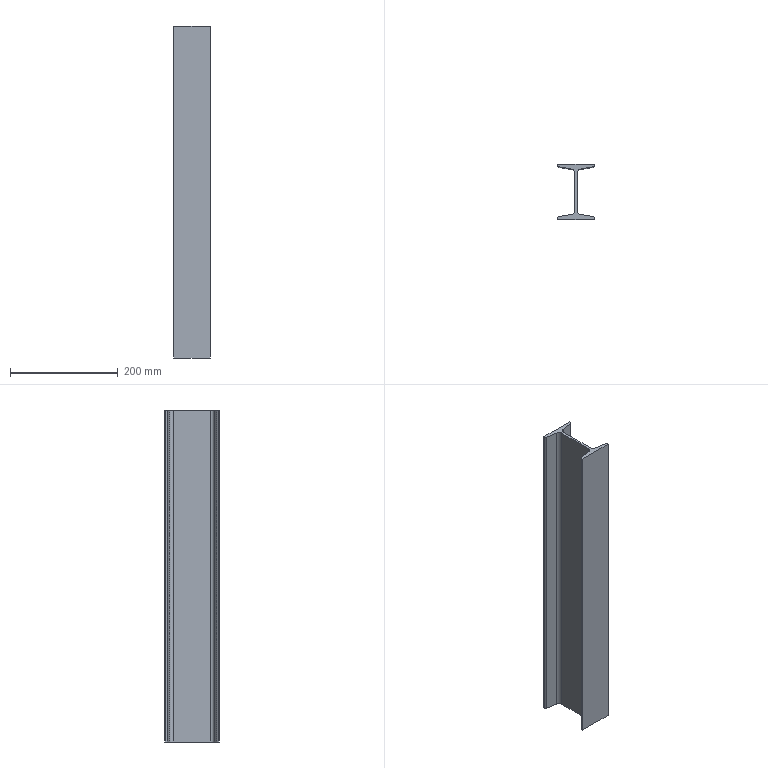Part | SolidWorks | features BaseBody 1 | 1 solid | 22 faces | box 67.6 x 101.6 x 617.6 mm | volume 858414 mm3 | plane 14 | cylinder 8 | commonest cylinder face diameters 5.6 x4 14.8 x4
STEP:
#1=CARTESIAN_POINT('',(9.458,64.672,0.));
#2=VERTEX_POINT('',#1);
#3=CARTESIAN_POINT('',(9.458,-5.208,0.));
#4=VERTEX_POINT('',#3);
#5=CARTESIAN_POINT('',(9.458,-5.208,0.));
#6=DIRECTION('',(0.,-1.,0.));
#7=VECTOR('',#6,1000.);
#8=LINE('',#5,#7);
#9=EDGE_CURVE('',#2,#4,#8,.T.);
#10=ORIENTED_EDGE('',*,*,#9,.T.);
#11=CARTESIAN_POINT('',(9.458,-5.208,617.6));
#12=VERTEX_POINT('',#11);
#13=CARTESIAN_POINT('',(9.458,-5.208,0.));
#14=DIRECTION('',(0.,0.,1.));
#15=VECTOR('',#14,1000.);
#16=LINE('',#13,#15);
#17=EDGE_CURVE('',#4,#12,#16,.T.);
#18=ORIENTED_EDGE('',*,*,#17,.T.);
#19=CARTESIAN_POINT('',(9.458,64.672,617.6));
#20=VERTEX_POINT('',#19);
#21=CARTESIAN_POINT('',(9.458,-5.208,617.6));
#22=DIRECTION('',(0.,1.,0.));
#23=VECTOR('',#22,1000.);
#24=LINE('',#21,#23);
#25=EDGE_CURVE('',#12,#20,#24,.T.);
#26=ORIENTED_EDGE('',*,*,#25,.T.);
#27=CARTESIAN_POINT('',(9.458,64.672,0.));
#28=DIRECTION('',(0.,0.,-1.));
#29=VECTOR('',#28,1000.);
#30=LINE('',#27,#29);
#31=EDGE_CURVE('',#20,#2,#30,.T.);
#32=ORIENTED_EDGE('',*,*,#31,.T.);
#33=EDGE_LOOP('',(#10,#18,#26,#32));
#34=FACE_OUTER_BOUND('',#33,.T.);
#35=CARTESIAN_POINT('',(9.458,-5.208,0.));
#36=DIRECTION('',(-1.,0.,0.));
#37=DIRECTION('',(0.,0.,1.));
#38=AXIS2_PLACEMENT_3D('',#35,#36,#37);
#39=PLANE('',#38);
#40=ADVANCED_FACE('',(#34),#39,.T.);
#41=ORIENTED_EDGE('',*,*,#17,.F.);
#42=CARTESIAN_POINT('',(3.279,-12.506,0.));
#43=VERTEX_POINT('',#42);
#44=CARTESIAN_POINT('',(2.058,-5.208,0.));
#45=DIRECTION('',(0.,0.,1.));
#46=DIRECTION('',(1.,0.,0.));
#47=AXIS2_PLACEMENT_3D('',#44,#45,#46);
#48=CIRCLE('',#47,7.4);
#49=EDGE_CURVE('',#43,#4,#48,.T.);
#50=ORIENTED_EDGE('',*,*,#49,.F.);
#51=CARTESIAN_POINT('',(3.279,-12.506,617.6));
#52=VERTEX_POINT('',#51);
#53=CARTESIAN_POINT('',(3.279,-12.506,0.));
#54=DIRECTION('',(0.,0.,-1.));
#55=VECTOR('',#54,1000.);
#56=LINE('',#53,#55);
#57=EDGE_CURVE('',#52,#43,#56,.T.);
#58=ORIENTED_EDGE('',*,*,#57,.F.);
#59=CARTESIAN_POINT('',(2.058,-5.208,617.6));
#60=DIRECTION('',(0.,0.,-1.));
#61=DIRECTION('',(1.,0.,0.));
#62=AXIS2_PLACEMENT_3D('',#59,#60,#61);
#63=CIRCLE('',#62,7.4);
#64=EDGE_CURVE('',#12,#52,#63,.T.);
#65=ORIENTED_EDGE('',*,*,#64,.F.);
#66=EDGE_LOOP('',(#41,#50,#58,#65));
#67=FACE_OUTER_BOUND('',#66,.T.);
#68=CARTESIAN_POINT('',(2.058,-5.208,0.));
#69=DIRECTION('',(0.,0.,1.));
#70=DIRECTION('',(1.,0.,0.));
#71=AXIS2_PLACEMENT_3D('',#68,#69,#70);
#72=CYLINDRICAL_SURFACE('',#71,7.4);
#73=ADVANCED_FACE('',(#67),#72,.F.);
#74=CARTESIAN_POINT('',(-19.604,-16.336,0.));
#75=VERTEX_POINT('',#74);
#76=CARTESIAN_POINT('',(-21.942,-19.097,0.));
#77=VERTEX_POINT('',#76);
#78=CARTESIAN_POINT('',(-19.142,-19.097,0.));
#79=DIRECTION('',(0.,0.,1.));
#80=DIRECTION('',(1.,0.,0.));
#81=AXIS2_PLACEMENT_3D('',#78,#79,#80);
#82=CIRCLE('',#81,2.8);
#83=EDGE_CURVE('',#75,#77,#82,.T.);
#84=ORIENTED_EDGE('',*,*,#83,.F.);
#85=CARTESIAN_POINT('',(3.279,-12.506,0.));
#86=DIRECTION('',(-0.9863,-0.165,0.));
#87=VECTOR('',#86,1000.);
#88=LINE('',#85,#87);
#89=EDGE_CURVE('',#43,#75,#88,.T.);
#90=ORIENTED_EDGE('',*,*,#89,.F.);
#91=ORIENTED_EDGE('',*,*,#49,.T.);
#92=ORIENTED_EDGE('',*,*,#9,.F.);
#93=CARTESIAN_POINT('',(3.279,71.971,0.));
#94=VERTEX_POINT('',#93);
#95=CARTESIAN_POINT('',(2.058,64.672,0.));
#96=DIRECTION('',(0.,0.,-1.));
#97=DIRECTION('',(1.,0.,0.));
#98=AXIS2_PLACEMENT_3D('',#95,#96,#97);
#99=CIRCLE('',#98,7.4);
#100=EDGE_CURVE('',#94,#2,#99,.T.);
#101=ORIENTED_EDGE('',*,*,#100,.F.);
#102=CARTESIAN_POINT('',(-19.604,75.8,0.));
#103=VERTEX_POINT('',#102);
#104=CARTESIAN_POINT('',(-19.604,75.8,0.));
#105=DIRECTION('',(0.9863,-0.165,0.));
#106=VECTOR('',#105,1000.);
#107=LINE('',#104,#106);
#108=EDGE_CURVE('',#103,#94,#107,.T.);
#109=ORIENTED_EDGE('',*,*,#108,.F.);
#110=CARTESIAN_POINT('',(-21.942,78.562,0.));
#111=VERTEX_POINT('',#110);
#112=CARTESIAN_POINT('',(-19.142,78.562,0.));
#113=DIRECTION('',(0.,0.,1.));
#114=DIRECTION('',(1.,0.,0.));
#115=AXIS2_PLACEMENT_3D('',#112,#113,#114);
#116=CIRCLE('',#115,2.8);
#117=EDGE_CURVE('',#111,#103,#116,.T.);
#118=ORIENTED_EDGE('',*,*,#117,.F.);
#119=CARTESIAN_POINT('',(-21.942,80.532,0.));
#120=VERTEX_POINT('',#119);
#121=CARTESIAN_POINT('',(-21.942,29.732,0.));
#122=DIRECTION('',(0.,-1.,0.));
#123=VECTOR('',#122,1000.);
#124=LINE('',#121,#123);
#125=EDGE_CURVE('',#120,#111,#124,.T.);
#126=ORIENTED_EDGE('',*,*,#125,.F.);
#127=CARTESIAN_POINT('',(45.658,80.532,0.));
#128=VERTEX_POINT('',#127);
#129=CARTESIAN_POINT('',(11.858,80.532,0.));
#130=DIRECTION('',(-1.,0.,0.));
#131=VECTOR('',#130,1000.);
#132=LINE('',#129,#131);
#133=EDGE_CURVE('',#128,#120,#132,.T.);
#134=ORIENTED_EDGE('',*,*,#133,.F.);
#135=CARTESIAN_POINT('',(45.658,78.562,0.));
#136=VERTEX_POINT('',#135);
#137=CARTESIAN_POINT('',(45.658,29.732,0.));
#138=DIRECTION('',(0.,1.,0.));
#139=VECTOR('',#138,1000.);
#140=LINE('',#137,#139);
#141=EDGE_CURVE('',#136,#128,#140,.T.);
#142=ORIENTED_EDGE('',*,*,#141,.F.);
#143=CARTESIAN_POINT('',(43.32,75.8,0.));
#144=VERTEX_POINT('',#143);
#145=CARTESIAN_POINT('',(42.858,78.562,0.));
#146=DIRECTION('',(0.,0.,1.));
#147=DIRECTION('',(1.,0.,0.));
#148=AXIS2_PLACEMENT_3D('',#145,#146,#147);
#149=CIRCLE('',#148,2.8);
#150=EDGE_CURVE('',#144,#136,#149,.T.);
#151=ORIENTED_EDGE('',*,*,#150,.F.);
#152=CARTESIAN_POINT('',(20.437,71.971,0.));
#153=VERTEX_POINT('',#152);
#154=CARTESIAN_POINT('',(20.437,71.971,0.));
#155=DIRECTION('',(0.9863,0.165,0.));
#156=VECTOR('',#155,1000.);
#157=LINE('',#154,#156);
#158=EDGE_CURVE('',#153,#144,#157,.T.);
#159=ORIENTED_EDGE('',*,*,#158,.F.);
#160=CARTESIAN_POINT('',(14.258,64.672,0.));
#161=VERTEX_POINT('',#160);
#162=CARTESIAN_POINT('',(21.658,64.672,0.));
#163=DIRECTION('',(0.,0.,-1.));
#164=DIRECTION('',(1.,0.,0.));
#165=AXIS2_PLACEMENT_3D('',#162,#163,#164);
#166=CIRCLE('',#165,7.4);
#167=EDGE_CURVE('',#161,#153,#166,.T.);
#168=ORIENTED_EDGE('',*,*,#167,.F.);
#169=CARTESIAN_POINT('',(14.258,-5.208,0.));
#170=VERTEX_POINT('',#169);
#171=CARTESIAN_POINT('',(14.258,29.732,0.));
#172=DIRECTION('',(0.,1.,0.));
#173=VECTOR('',#172,1000.);
#174=LINE('',#171,#173);
#175=EDGE_CURVE('',#170,#161,#174,.T.);
#176=ORIENTED_EDGE('',*,*,#175,.F.);
#177=CARTESIAN_POINT('',(20.437,-12.506,0.));
#178=VERTEX_POINT('',#177);
#179=CARTESIAN_POINT('',(21.658,-5.208,0.));
#180=DIRECTION('',(0.,0.,-1.));
#181=DIRECTION('',(1.,0.,0.));
#182=AXIS2_PLACEMENT_3D('',#179,#180,#181);
#183=CIRCLE('',#182,7.4);
#184=EDGE_CURVE('',#178,#170,#183,.T.);
#185=ORIENTED_EDGE('',*,*,#184,.F.);
#186=CARTESIAN_POINT('',(43.32,-16.336,0.));
#187=VERTEX_POINT('',#186);
#188=CARTESIAN_POINT('',(43.32,-16.336,0.));
#189=DIRECTION('',(-0.9863,0.165,0.));
#190=VECTOR('',#189,1000.);
#191=LINE('',#188,#190);
#192=EDGE_CURVE('',#187,#178,#191,.T.);
#193=ORIENTED_EDGE('',*,*,#192,.F.);
#194=CARTESIAN_POINT('',(45.658,-19.097,0.));
#195=VERTEX_POINT('',#194);
#196=CARTESIAN_POINT('',(42.858,-19.097,0.));
#197=DIRECTION('',(0.,0.,1.));
#198=DIRECTION('',(1.,0.,0.));
#199=AXIS2_PLACEMENT_3D('',#196,#197,#198);
#200=CIRCLE('',#199,2.8);
#201=EDGE_CURVE('',#195,#187,#200,.T.);
#202=ORIENTED_EDGE('',*,*,#201,.F.);
#203=CARTESIAN_POINT('',(45.658,-21.068,0.));
#204=VERTEX_POINT('',#203);
#205=CARTESIAN_POINT('',(45.658,29.732,0.));
#206=DIRECTION('',(0.,1.,0.));
#207=VECTOR('',#206,1000.);
#208=LINE('',#205,#207);
#209=EDGE_CURVE('',#204,#195,#208,.T.);
#210=ORIENTED_EDGE('',*,*,#209,.F.);
#211=CARTESIAN_POINT('',(-21.942,-21.068,0.));
#212=VERTEX_POINT('',#211);
#213=CARTESIAN_POINT('',(11.858,-21.068,0.));
#214=DIRECTION('',(1.,0.,0.));
#215=VECTOR('',#214,1000.);
#216=LINE('',#213,#215);
#217=EDGE_CURVE('',#212,#204,#216,.T.);
#218=ORIENTED_EDGE('',*,*,#217,.F.);
#219=CARTESIAN_POINT('',(-21.942,29.732,0.));
#220=DIRECTION('',(0.,-1.,0.));
#221=VECTOR('',#220,1000.);
#222=LINE('',#219,#221);
#223=EDGE_CURVE('',#77,#212,#222,.T.);
#224=ORIENTED_EDGE('',*,*,#223,.F.);
#225=EDGE_LOOP('',(#84,#90,#91,#92,#101,#109,#118,#126,#134,#142,#151,#159,#168,#176,#185,#193,#202,#210,#218,#224));
#226=FACE_OUTER_BOUND('',#225,.T.);
#227=CARTESIAN_POINT('',(11.858,29.732,0.));
#228=DIRECTION('',(0.,0.,1.));
#229=DIRECTION('',(1.,0.,0.));
#230=AXIS2_PLACEMENT_3D('',#227,#228,#229);
#231=PLANE('',#230);
#232=ADVANCED_FACE('',(#226),#231,.F.);
#233=CARTESIAN_POINT('',(3.279,71.971,617.6));
#234=VERTEX_POINT('',#233);
#235=CARTESIAN_POINT('',(3.279,71.971,0.));
#236=DIRECTION('',(0.,0.,1.));
#237=VECTOR('',#236,1000.);
#238=LINE('',#235,#237);
#239=EDGE_CURVE('',#94,#234,#238,.T.);
#240=ORIENTED_EDGE('',*,*,#239,.F.);
#241=ORIENTED_EDGE('',*,*,#100,.T.);
#242=ORIENTED_EDGE('',*,*,#31,.F.);
#243=CARTESIAN_POINT('',(2.058,64.672,617.6));
#244=DIRECTION('',(0.,0.,-1.));
#245=DIRECTION('',(1.,0.,0.));
#246=AXIS2_PLACEMENT_3D('',#243,#244,#245);
#247=CIRCLE('',#246,7.4);
#248=EDGE_CURVE('',#234,#20,#247,.T.);
#249=ORIENTED_EDGE('',*,*,#248,.F.);
#250=EDGE_LOOP('',(#240,#241,#242,#249));
#251=FACE_OUTER_BOUND('',#250,.T.);
#252=CARTESIAN_POINT('',(2.058,64.672,0.));
#253=DIRECTION('',(0.,0.,1.));
#254=DIRECTION('',(1.,0.,0.));
#255=AXIS2_PLACEMENT_3D('',#252,#253,#254);
#256=CYLINDRICAL_SURFACE('',#255,7.4);
#257=ADVANCED_FACE('',(#251),#256,.F.);
#258=ORIENTED_EDGE('',*,*,#64,.T.);
#259=CARTESIAN_POINT('',(-19.604,-16.336,617.6));
#260=VERTEX_POINT('',#259);
#261=CARTESIAN_POINT('',(3.279,-12.506,617.6));
#262=DIRECTION('',(-0.9863,-0.165,0.));
#263=VECTOR('',#262,1000.);
#264=LINE('',#261,#263);
#265=EDGE_CURVE('',#52,#260,#264,.T.);
#266=ORIENTED_EDGE('',*,*,#265,.T.);
#267=CARTESIAN_POINT('',(-21.942,-19.097,617.6));
#268=VERTEX_POINT('',#267);
#269=CARTESIAN_POINT('',(-19.142,-19.097,617.6));
#270=DIRECTION('',(0.,0.,1.));
#271=DIRECTION('',(1.,0.,0.));
#272=AXIS2_PLACEMENT_3D('',#269,#270,#271);
#273=CIRCLE('',#272,2.8);
#274=EDGE_CURVE('',#260,#268,#273,.T.);
#275=ORIENTED_EDGE('',*,*,#274,.T.);
#276=CARTESIAN_POINT('',(-21.942,-21.068,617.6));
#277=VERTEX_POINT('',#276);
#278=CARTESIAN_POINT('',(-21.942,29.732,617.6));
#279=DIRECTION('',(0.,-1.,0.));
#280=VECTOR('',#279,1000.);
#281=LINE('',#278,#280);
#282=EDGE_CURVE('',#268,#277,#281,.T.);
#283=ORIENTED_EDGE('',*,*,#282,.T.);
#284=CARTESIAN_POINT('',(45.658,-21.068,617.6));
#285=VERTEX_POINT('',#284);
#286=CARTESIAN_POINT('',(11.858,-21.068,617.6));
#287=DIRECTION('',(1.,0.,0.));
#288=VECTOR('',#287,1000.);
#289=LINE('',#286,#288);
#290=EDGE_CURVE('',#277,#285,#289,.T.);
#291=ORIENTED_EDGE('',*,*,#290,.T.);
#292=CARTESIAN_POINT('',(45.658,-19.097,617.6));
#293=VERTEX_POINT('',#292);
#294=CARTESIAN_POINT('',(45.658,29.732,617.6));
#295=DIRECTION('',(0.,1.,0.));
#296=VECTOR('',#295,1000.);
#297=LINE('',#294,#296);
#298=EDGE_CURVE('',#285,#293,#297,.T.);
#299=ORIENTED_EDGE('',*,*,#298,.T.);
#300=CARTESIAN_POINT('',(43.32,-16.336,617.6));
#301=VERTEX_POINT('',#300);
#302=CARTESIAN_POINT('',(42.858,-19.097,617.6));
#303=DIRECTION('',(0.,0.,1.));
#304=DIRECTION('',(1.,0.,0.));
#305=AXIS2_PLACEMENT_3D('',#302,#303,#304);
#306=CIRCLE('',#305,2.8);
#307=EDGE_CURVE('',#293,#301,#306,.T.);
#308=ORIENTED_EDGE('',*,*,#307,.T.);
#309=CARTESIAN_POINT('',(20.437,-12.506,617.6));
#310=VERTEX_POINT('',#309);
#311=CARTESIAN_POINT('',(43.32,-16.336,617.6));
#312=DIRECTION('',(-0.9863,0.165,0.));
#313=VECTOR('',#312,1000.);
#314=LINE('',#311,#313);
#315=EDGE_CURVE('',#301,#310,#314,.T.);
#316=ORIENTED_EDGE('',*,*,#315,.T.);
#317=CARTESIAN_POINT('',(14.258,-5.208,617.6));
#318=VERTEX_POINT('',#317);
#319=CARTESIAN_POINT('',(21.658,-5.208,617.6));
#320=DIRECTION('',(0.,0.,-1.));
#321=DIRECTION('',(1.,0.,0.));
#322=AXIS2_PLACEMENT_3D('',#319,#320,#321);
#323=CIRCLE('',#322,7.4);
#324=EDGE_CURVE('',#310,#318,#323,.T.);
#325=ORIENTED_EDGE('',*,*,#324,.T.);
#326=CARTESIAN_POINT('',(14.258,64.672,617.6));
#327=VERTEX_POINT('',#326);
#328=CARTESIAN_POINT('',(14.258,29.732,617.6));
#329=DIRECTION('',(0.,1.,0.));
#330=VECTOR('',#329,1000.);
#331=LINE('',#328,#330);
#332=EDGE_CURVE('',#318,#327,#331,.T.);
#333=ORIENTED_EDGE('',*,*,#332,.T.);
#334=CARTESIAN_POINT('',(20.437,71.971,617.6));
#335=VERTEX_POINT('',#334);
#336=CARTESIAN_POINT('',(21.658,64.672,617.6));
#337=DIRECTION('',(0.,0.,-1.));
#338=DIRECTION('',(1.,0.,0.));
#339=AXIS2_PLACEMENT_3D('',#336,#337,#338);
#340=CIRCLE('',#339,7.4);
#341=EDGE_CURVE('',#327,#335,#340,.T.);
#342=ORIENTED_EDGE('',*,*,#341,.T.);
#343=CARTESIAN_POINT('',(43.32,75.8,617.6));
#344=VERTEX_POINT('',#343);
#345=CARTESIAN_POINT('',(20.437,71.971,617.6));
#346=DIRECTION('',(0.9863,0.165,0.));
#347=VECTOR('',#346,1000.);
#348=LINE('',#345,#347);
#349=EDGE_CURVE('',#335,#344,#348,.T.);
#350=ORIENTED_EDGE('',*,*,#349,.T.);
#351=CARTESIAN_POINT('',(45.658,78.562,617.6));
#352=VERTEX_POINT('',#351);
#353=CARTESIAN_POINT('',(42.858,78.562,617.6));
#354=DIRECTION('',(0.,0.,1.));
#355=DIRECTION('',(1.,0.,0.));
#356=AXIS2_PLACEMENT_3D('',#353,#354,#355);
#357=CIRCLE('',#356,2.8);
#358=EDGE_CURVE('',#344,#352,#357,.T.);
#359=ORIENTED_EDGE('',*,*,#358,.T.);
#360=CARTESIAN_POINT('',(45.658,80.532,617.6));
#361=VERTEX_POINT('',#360);
#362=CARTESIAN_POINT('',(45.658,29.732,617.6));
#363=DIRECTION('',(0.,1.,0.));
#364=VECTOR('',#363,1000.);
#365=LINE('',#362,#364);
#366=EDGE_CURVE('',#352,#361,#365,.T.);
#367=ORIENTED_EDGE('',*,*,#366,.T.);
#368=CARTESIAN_POINT('',(-21.942,80.532,617.6));
#369=VERTEX_POINT('',#368);
#370=CARTESIAN_POINT('',(11.858,80.532,617.6));
#371=DIRECTION('',(-1.,0.,0.));
#372=VECTOR('',#371,1000.);
#373=LINE('',#370,#372);
#374=EDGE_CURVE('',#361,#369,#373,.T.);
#375=ORIENTED_EDGE('',*,*,#374,.T.);
#376=CARTESIAN_POINT('',(-21.942,78.562,617.6));
#377=VERTEX_POINT('',#376);
#378=CARTESIAN_POINT('',(-21.942,29.732,617.6));
#379=DIRECTION('',(0.,-1.,0.));
#380=VECTOR('',#379,1000.);
#381=LINE('',#378,#380);
#382=EDGE_CURVE('',#369,#377,#381,.T.);
#383=ORIENTED_EDGE('',*,*,#382,.T.);
#384=CARTESIAN_POINT('',(-19.604,75.8,617.6));
#385=VERTEX_POINT('',#384);
#386=CARTESIAN_POINT('',(-19.142,78.562,617.6));
#387=DIRECTION('',(0.,0.,1.));
#388=DIRECTION('',(1.,0.,0.));
#389=AXIS2_PLACEMENT_3D('',#386,#387,#388);
#390=CIRCLE('',#389,2.8);
#391=EDGE_CURVE('',#377,#385,#390,.T.);
#392=ORIENTED_EDGE('',*,*,#391,.T.);
#393=CARTESIAN_POINT('',(-19.604,75.8,617.6));
#394=DIRECTION('',(0.9863,-0.165,0.));
#395=VECTOR('',#394,1000.);
#396=LINE('',#393,#395);
#397=EDGE_CURVE('',#385,#234,#396,.T.);
#398=ORIENTED_EDGE('',*,*,#397,.T.);
#399=ORIENTED_EDGE('',*,*,#248,.T.);
#400=ORIENTED_EDGE('',*,*,#25,.F.);
#401=EDGE_LOOP('',(#258,#266,#275,#283,#291,#299,#308,#316,#325,#333,#342,#350,#359,#367,#375,#383,#392,#398,#399,#400));
#402=FACE_OUTER_BOUND('',#401,.T.);
#403=CARTESIAN_POINT('',(11.858,29.732,617.6));
#404=DIRECTION('',(0.,0.,1.));
#405=DIRECTION('',(1.,0.,0.));
#406=AXIS2_PLACEMENT_3D('',#403,#404,#405);
#407=PLANE('',#406);
#408=ADVANCED_FACE('',(#402),#407,.T.);
#409=ORIENTED_EDGE('',*,*,#89,.T.);
#410=CARTESIAN_POINT('',(-19.604,-16.336,0.));
#411=DIRECTION('',(0.,0.,1.));
#412=VECTOR('',#411,1000.);
#413=LINE('',#410,#412);
#414=EDGE_CURVE('',#75,#260,#413,.T.);
#415=ORIENTED_EDGE('',*,*,#414,.T.);
#416=ORIENTED_EDGE('',*,*,#265,.F.);
#417=ORIENTED_EDGE('',*,*,#57,.T.);
#418=EDGE_LOOP('',(#409,#415,#416,#417));
#419=FACE_OUTER_BOUND('',#418,.T.);
#420=CARTESIAN_POINT('',(-19.604,-16.336,0.));
#421=DIRECTION('',(-0.165,0.9863,0.));
#422=DIRECTION('',(-0.9863,-0.165,0.));
#423=AXIS2_PLACEMENT_3D('',#420,#421,#422);
#424=PLANE('',#423);
#425=ADVANCED_FACE('',(#419),#424,.T.);
#426=ORIENTED_EDGE('',*,*,#223,.T.);
#427=CARTESIAN_POINT('',(-21.942,-21.068,0.));
#428=DIRECTION('',(0.,0.,1.));
#429=VECTOR('',#428,1000.);
#430=LINE('',#427,#429);
#431=EDGE_CURVE('',#212,#277,#430,.T.);
#432=ORIENTED_EDGE('',*,*,#431,.T.);
#433=ORIENTED_EDGE('',*,*,#282,.F.);
#434=CARTESIAN_POINT('',(-21.942,-19.097,0.));
#435=DIRECTION('',(0.,0.,-1.));
#436=VECTOR('',#435,1000.);
#437=LINE('',#434,#436);
#438=EDGE_CURVE('',#268,#77,#437,.T.);
#439=ORIENTED_EDGE('',*,*,#438,.T.);
#440=EDGE_LOOP('',(#426,#432,#433,#439));
#441=FACE_OUTER_BOUND('',#440,.T.);
#442=CARTESIAN_POINT('',(-21.942,-21.068,0.));
#443=DIRECTION('',(-1.,0.,0.));
#444=DIRECTION('',(0.,0.,1.));
#445=AXIS2_PLACEMENT_3D('',#442,#443,#444);
#446=PLANE('',#445);
#447=ADVANCED_FACE('',(#441),#446,.T.);
#448=ORIENTED_EDGE('',*,*,#83,.T.);
#449=ORIENTED_EDGE('',*,*,#438,.F.);
#450=ORIENTED_EDGE('',*,*,#274,.F.);
#451=ORIENTED_EDGE('',*,*,#414,.F.);
#452=EDGE_LOOP('',(#448,#449,#450,#451));
#453=FACE_OUTER_BOUND('',#452,.T.);
#454=CARTESIAN_POINT('',(-19.142,-19.097,0.));
#455=DIRECTION('',(0.,0.,1.));
#456=DIRECTION('',(1.,0.,0.));
#457=AXIS2_PLACEMENT_3D('',#454,#455,#456);
#458=CYLINDRICAL_SURFACE('',#457,2.8);
#459=ADVANCED_FACE('',(#453),#458,.T.);
#460=ORIENTED_EDGE('',*,*,#108,.T.);
#461=ORIENTED_EDGE('',*,*,#239,.T.);
#462=ORIENTED_EDGE('',*,*,#397,.F.);
#463=CARTESIAN_POINT('',(-19.604,75.8,0.));
#464=DIRECTION('',(0.,0.,-1.));
#465=VECTOR('',#464,1000.);
#466=LINE('',#463,#465);
#467=EDGE_CURVE('',#385,#103,#466,.T.);
#468=ORIENTED_EDGE('',*,*,#467,.T.);
#469=EDGE_LOOP('',(#460,#461,#462,#468));
#470=FACE_OUTER_BOUND('',#469,.T.);
#471=CARTESIAN_POINT('',(3.279,71.971,0.));
#472=DIRECTION('',(-0.165,-0.9863,0.));
#473=DIRECTION('',(0.9863,-0.165,0.));
#474=AXIS2_PLACEMENT_3D('',#471,#472,#473);
#475=PLANE('',#474);
#476=ADVANCED_FACE('',(#470),#475,.T.);
#477=ORIENTED_EDGE('',*,*,#117,.T.);
#478=ORIENTED_EDGE('',*,*,#467,.F.);
#479=ORIENTED_EDGE('',*,*,#391,.F.);
#480=CARTESIAN_POINT('',(-21.942,78.562,0.));
#481=DIRECTION('',(0.,0.,-1.));
#482=VECTOR('',#481,1000.);
#483=LINE('',#480,#482);
#484=EDGE_CURVE('',#377,#111,#483,.T.);
#485=ORIENTED_EDGE('',*,*,#484,.T.);
#486=EDGE_LOOP('',(#477,#478,#479,#485));
#487=FACE_OUTER_BOUND('',#486,.T.);
#488=CARTESIAN_POINT('',(-19.142,78.562,0.));
#489=DIRECTION('',(0.,0.,1.));
#490=DIRECTION('',(1.,0.,0.));
#491=AXIS2_PLACEMENT_3D('',#488,#489,#490);
#492=CYLINDRICAL_SURFACE('',#491,2.8);
#493=ADVANCED_FACE('',(#487),#492,.T.);
#494=ORIENTED_EDGE('',*,*,#125,.T.);
#495=ORIENTED_EDGE('',*,*,#484,.F.);
#496=ORIENTED_EDGE('',*,*,#382,.F.);
#497=CARTESIAN_POINT('',(-21.942,80.532,0.));
#498=DIRECTION('',(0.,0.,-1.));
#499=VECTOR('',#498,1000.);
#500=LINE('',#497,#499);
#501=EDGE_CURVE('',#369,#120,#500,.T.);
#502=ORIENTED_EDGE('',*,*,#501,.T.);
#503=EDGE_LOOP('',(#494,#495,#496,#502));
#504=FACE_OUTER_BOUND('',#503,.T.);
#505=CARTESIAN_POINT('',(-21.942,78.562,0.));
#506=DIRECTION('',(-1.,0.,0.));
#507=DIRECTION('',(0.,0.,1.));
#508=AXIS2_PLACEMENT_3D('',#505,#506,#507);
#509=PLANE('',#508);
#510=ADVANCED_FACE('',(#504),#509,.T.);
#511=ORIENTED_EDGE('',*,*,#133,.T.);
#512=ORIENTED_EDGE('',*,*,#501,.F.);
#513=ORIENTED_EDGE('',*,*,#374,.F.);
#514=CARTESIAN_POINT('',(45.658,80.532,0.));
#515=DIRECTION('',(0.,0.,-1.));
#516=VECTOR('',#515,1000.);
#517=LINE('',#514,#516);
#518=EDGE_CURVE('',#361,#128,#517,.T.);
#519=ORIENTED_EDGE('',*,*,#518,.T.);
#520=EDGE_LOOP('',(#511,#512,#513,#519));
#521=FACE_OUTER_BOUND('',#520,.T.);
#522=CARTESIAN_POINT('',(-21.942,80.532,0.));
#523=DIRECTION('',(0.,1.,0.));
#524=DIRECTION('',(0.,0.,1.));
#525=AXIS2_PLACEMENT_3D('',#522,#523,#524);
#526=PLANE('',#525);
#527=ADVANCED_FACE('',(#521),#526,.T.);
#528=ORIENTED_EDGE('',*,*,#141,.T.);
#529=ORIENTED_EDGE('',*,*,#518,.F.);
#530=ORIENTED_EDGE('',*,*,#366,.F.);
#531=CARTESIAN_POINT('',(45.658,78.562,0.));
#532=DIRECTION('',(0.,0.,-1.));
#533=VECTOR('',#532,1000.);
#534=LINE('',#531,#533);
#535=EDGE_CURVE('',#352,#136,#534,.T.);
#536=ORIENTED_EDGE('',*,*,#535,.T.);
#537=EDGE_LOOP('',(#528,#529,#530,#536));
#538=FACE_OUTER_BOUND('',#537,.T.);
#539=CARTESIAN_POINT('',(45.658,80.532,0.));
#540=DIRECTION('',(1.,0.,0.));
#541=DIRECTION('',(0.,0.,-1.));
#542=AXIS2_PLACEMENT_3D('',#539,#540,#541);
#543=PLANE('',#542);
#544=ADVANCED_FACE('',(#538),#543,.T.);
#545=ORIENTED_EDGE('',*,*,#150,.T.);
#546=ORIENTED_EDGE('',*,*,#535,.F.);
#547=ORIENTED_EDGE('',*,*,#358,.F.);
#548=CARTESIAN_POINT('',(43.32,75.8,0.));
#549=DIRECTION('',(0.,0.,-1.));
#550=VECTOR('',#549,1000.);
#551=LINE('',#548,#550);
#552=EDGE_CURVE('',#344,#144,#551,.T.);
#553=ORIENTED_EDGE('',*,*,#552,.T.);
#554=EDGE_LOOP('',(#545,#546,#547,#553));
#555=FACE_OUTER_BOUND('',#554,.T.);
#556=CARTESIAN_POINT('',(42.858,78.562,0.));
#557=DIRECTION('',(0.,0.,1.));
#558=DIRECTION('',(1.,0.,0.));
#559=AXIS2_PLACEMENT_3D('',#556,#557,#558);
#560=CYLINDRICAL_SURFACE('',#559,2.8);
#561=ADVANCED_FACE('',(#555),#560,.T.);
#562=ORIENTED_EDGE('',*,*,#158,.T.);
#563=ORIENTED_EDGE('',*,*,#552,.F.);
#564=ORIENTED_EDGE('',*,*,#349,.F.);
#565=CARTESIAN_POINT('',(20.437,71.971,0.));
#566=DIRECTION('',(0.,0.,-1.));
#567=VECTOR('',#566,1000.);
#568=LINE('',#565,#567);
#569=EDGE_CURVE('',#335,#153,#568,.T.);
#570=ORIENTED_EDGE('',*,*,#569,.T.);
#571=EDGE_LOOP('',(#562,#563,#564,#570));
#572=FACE_OUTER_BOUND('',#571,.T.);
#573=CARTESIAN_POINT('',(43.32,75.8,0.));
#574=DIRECTION('',(0.165,-0.9863,0.));
#575=DIRECTION('',(0.9863,0.165,0.));
#576=AXIS2_PLACEMENT_3D('',#573,#574,#575);
#577=PLANE('',#576);
#578=ADVANCED_FACE('',(#572),#577,.T.);
#579=CARTESIAN_POINT('',(14.258,64.672,0.));
#580=DIRECTION('',(0.,0.,1.));
#581=VECTOR('',#580,1000.);
#582=LINE('',#579,#581);
#583=EDGE_CURVE('',#161,#327,#582,.T.);
#584=ORIENTED_EDGE('',*,*,#583,.F.);
#585=ORIENTED_EDGE('',*,*,#167,.T.);
#586=ORIENTED_EDGE('',*,*,#569,.F.);
#587=ORIENTED_EDGE('',*,*,#341,.F.);
#588=EDGE_LOOP('',(#584,#585,#586,#587));
#589=FACE_OUTER_BOUND('',#588,.T.);
#590=CARTESIAN_POINT('',(21.658,64.672,0.));
#591=DIRECTION('',(0.,0.,1.));
#592=DIRECTION('',(1.,0.,0.));
#593=AXIS2_PLACEMENT_3D('',#590,#591,#592);
#594=CYLINDRICAL_SURFACE('',#593,7.4);
#595=ADVANCED_FACE('',(#589),#594,.F.);
#596=ORIENTED_EDGE('',*,*,#175,.T.);
#597=ORIENTED_EDGE('',*,*,#583,.T.);
#598=ORIENTED_EDGE('',*,*,#332,.F.);
#599=CARTESIAN_POINT('',(14.258,-5.208,0.));
#600=DIRECTION('',(0.,0.,-1.));
#601=VECTOR('',#600,1000.);
#602=LINE('',#599,#601);
#603=EDGE_CURVE('',#318,#170,#602,.T.);
#604=ORIENTED_EDGE('',*,*,#603,.T.);
#605=EDGE_LOOP('',(#596,#597,#598,#604));
#606=FACE_OUTER_BOUND('',#605,.T.);
#607=CARTESIAN_POINT('',(14.258,64.672,0.));
#608=DIRECTION('',(1.,0.,0.));
#609=DIRECTION('',(0.,0.,-1.));
#610=AXIS2_PLACEMENT_3D('',#607,#608,#609);
#611=PLANE('',#610);
#612=ADVANCED_FACE('',(#606),#611,.T.);
#613=CARTESIAN_POINT('',(20.437,-12.506,0.));
#614=DIRECTION('',(0.,0.,1.));
#615=VECTOR('',#614,1000.);
#616=LINE('',#613,#615);
#617=EDGE_CURVE('',#178,#310,#616,.T.);
#618=ORIENTED_EDGE('',*,*,#617,.F.);
#619=ORIENTED_EDGE('',*,*,#184,.T.);
#620=ORIENTED_EDGE('',*,*,#603,.F.);
#621=ORIENTED_EDGE('',*,*,#324,.F.);
#622=EDGE_LOOP('',(#618,#619,#620,#621));
#623=FACE_OUTER_BOUND('',#622,.T.);
#624=CARTESIAN_POINT('',(21.658,-5.208,0.));
#625=DIRECTION('',(0.,0.,1.));
#626=DIRECTION('',(1.,0.,0.));
#627=AXIS2_PLACEMENT_3D('',#624,#625,#626);
#628=CYLINDRICAL_SURFACE('',#627,7.4);
#629=ADVANCED_FACE('',(#623),#628,.F.);
#630=ORIENTED_EDGE('',*,*,#192,.T.);
#631=ORIENTED_EDGE('',*,*,#617,.T.);
#632=ORIENTED_EDGE('',*,*,#315,.F.);
#633=CARTESIAN_POINT('',(43.32,-16.336,0.));
#634=DIRECTION('',(0.,0.,-1.));
#635=VECTOR('',#634,1000.);
#636=LINE('',#633,#635);
#637=EDGE_CURVE('',#301,#187,#636,.T.);
#638=ORIENTED_EDGE('',*,*,#637,.T.);
#639=EDGE_LOOP('',(#630,#631,#632,#638));
#640=FACE_OUTER_BOUND('',#639,.T.);
#641=CARTESIAN_POINT('',(20.437,-12.506,0.));
#642=DIRECTION('',(0.165,0.9863,0.));
#643=DIRECTION('',(-0.9863,0.165,0.));
#644=AXIS2_PLACEMENT_3D('',#641,#642,#643);
#645=PLANE('',#644);
#646=ADVANCED_FACE('',(#640),#645,.T.);
#647=ORIENTED_EDGE('',*,*,#201,.T.);
#648=ORIENTED_EDGE('',*,*,#637,.F.);
#649=ORIENTED_EDGE('',*,*,#307,.F.);
#650=CARTESIAN_POINT('',(45.658,-19.097,0.));
#651=DIRECTION('',(0.,0.,-1.));
#652=VECTOR('',#651,1000.);
#653=LINE('',#650,#652);
#654=EDGE_CURVE('',#293,#195,#653,.T.);
#655=ORIENTED_EDGE('',*,*,#654,.T.);
#656=EDGE_LOOP('',(#647,#648,#649,#655));
#657=FACE_OUTER_BOUND('',#656,.T.);
#658=CARTESIAN_POINT('',(42.858,-19.097,0.));
#659=DIRECTION('',(0.,0.,1.));
#660=DIRECTION('',(1.,0.,0.));
#661=AXIS2_PLACEMENT_3D('',#658,#659,#660);
#662=CYLINDRICAL_SURFACE('',#661,2.8);
#663=ADVANCED_FACE('',(#657),#662,.T.);
#664=ORIENTED_EDGE('',*,*,#209,.T.);
#665=ORIENTED_EDGE('',*,*,#654,.F.);
#666=ORIENTED_EDGE('',*,*,#298,.F.);
#667=CARTESIAN_POINT('',(45.658,-21.068,0.));
#668=DIRECTION('',(0.,0.,-1.));
#669=VECTOR('',#668,1000.);
#670=LINE('',#667,#669);
#671=EDGE_CURVE('',#285,#204,#670,.T.);
#672=ORIENTED_EDGE('',*,*,#671,.T.);
#673=EDGE_LOOP('',(#664,#665,#666,#672));
#674=FACE_OUTER_BOUND('',#673,.T.);
#675=CARTESIAN_POINT('',(45.658,-19.097,0.));
#676=DIRECTION('',(1.,0.,0.));
#677=DIRECTION('',(0.,0.,-1.));
#678=AXIS2_PLACEMENT_3D('',#675,#676,#677);
#679=PLANE('',#678);
#680=ADVANCED_FACE('',(#674),#679,.T.);
#681=ORIENTED_EDGE('',*,*,#217,.T.);
#682=ORIENTED_EDGE('',*,*,#671,.F.);
#683=ORIENTED_EDGE('',*,*,#290,.F.);
#684=ORIENTED_EDGE('',*,*,#431,.F.);
#685=EDGE_LOOP('',(#681,#682,#683,#684));
#686=FACE_OUTER_BOUND('',#685,.T.);
#687=CARTESIAN_POINT('',(45.658,-21.068,0.));
#688=DIRECTION('',(0.,-1.,0.));
#689=DIRECTION('',(0.,0.,-1.));
#690=AXIS2_PLACEMENT_3D('',#687,#688,#689);
#691=PLANE('',#690);
#692=ADVANCED_FACE('',(#686),#691,.T.);
#693=CLOSED_SHELL('',(#40,#73,#232,#257,#408,#425,#447,#459,#476,#493,#510,#527,#544,#561,#578,#595,#612,#629,#646,#663,#680,#692));
#694=MANIFOLD_SOLID_BREP('',#693);
#695=CARTESIAN_POINT('',(0.,0.,0.));
#696=DIRECTION('',(0.,0.,1.));
#697=DIRECTION('',(1.,0.,0.));
#698=AXIS2_PLACEMENT_3D('',#695,#696,#697);
#699=(LENGTH_UNIT()NAMED_UNIT(*)SI_UNIT(.MILLI.,.METRE.));
#700=UNCERTAINTY_MEASURE_WITH_UNIT(LENGTH_MEASURE(0.00001),#699,'','');
#701=(NAMED_UNIT(*)PLANE_ANGLE_UNIT()SI_UNIT($,.RADIAN.));
#702=(NAMED_UNIT(*)SI_UNIT($,.STERADIAN.)SOLID_ANGLE_UNIT());
#703=(GEOMETRIC_REPRESENTATION_CONTEXT(3)GLOBAL_UNCERTAINTY_ASSIGNED_CONTEXT((#700))GLOBAL_UNIT_ASSIGNED_CONTEXT((#699,#701,#702))REPRESENTATION_CONTEXT('',''));
#704=ADVANCED_BREP_SHAPE_REPRESENTATION('',(#694,#698),#703);